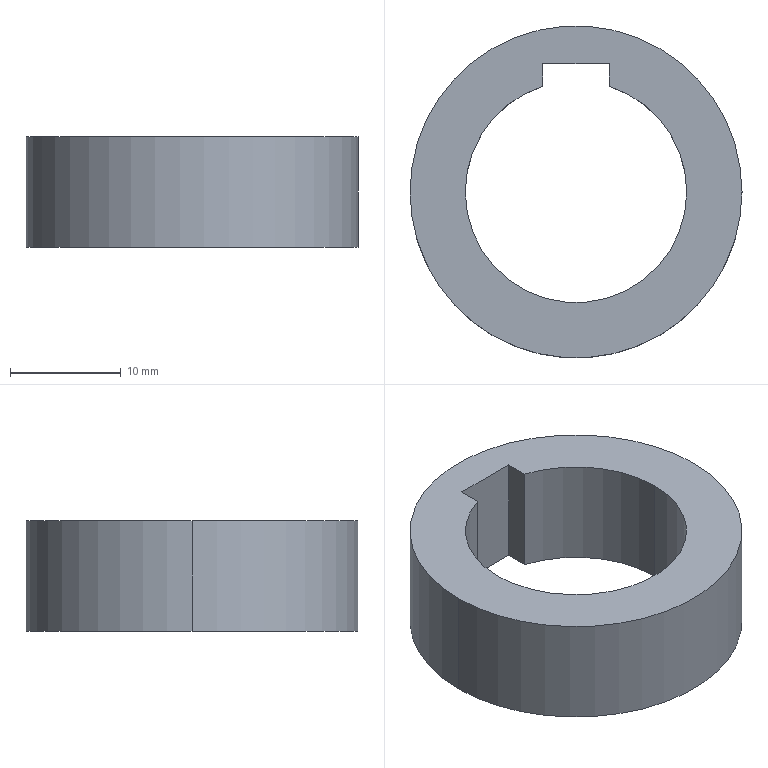Part | SolidWorks | features BaseBody 1 | 1 solid | 10 faces | box 30 x 30 x 10 mm | volume 3822 mm3 | cylinder 5 | plane 5 | commonest cylinder face diameters 20 x3 30 x2
STEP:
#1=CARTESIAN_POINT('',(10.,0.,10.));
#2=VERTEX_POINT('',#1);
#3=CARTESIAN_POINT('',(-10.,0.,10.));
#4=VERTEX_POINT('',#3);
#5=CARTESIAN_POINT('',(0.,0.,10.));
#6=DIRECTION('',(0.,0.,-1.));
#7=DIRECTION('',(-1.,0.,0.));
#8=AXIS2_PLACEMENT_3D('',#5,#6,#7);
#9=CIRCLE('',#8,10.);
#10=EDGE_CURVE('',#2,#4,#9,.T.);
#11=ORIENTED_EDGE('',*,*,#10,.F.);
#12=CARTESIAN_POINT('',(10.,0.,0.));
#13=VERTEX_POINT('',#12);
#14=CARTESIAN_POINT('',(10.,0.,0.));
#15=DIRECTION('',(0.,0.,-1.));
#16=VECTOR('',#15,1000.);
#17=LINE('',#14,#16);
#18=EDGE_CURVE('',#2,#13,#17,.T.);
#19=ORIENTED_EDGE('',*,*,#18,.T.);
#20=CARTESIAN_POINT('',(-10.,0.,0.));
#21=VERTEX_POINT('',#20);
#22=CARTESIAN_POINT('',(0.,0.,0.));
#23=DIRECTION('',(0.,0.,1.));
#24=DIRECTION('',(-1.,0.,0.));
#25=AXIS2_PLACEMENT_3D('',#22,#23,#24);
#26=CIRCLE('',#25,10.);
#27=EDGE_CURVE('',#21,#13,#26,.T.);
#28=ORIENTED_EDGE('',*,*,#27,.F.);
#29=CARTESIAN_POINT('',(-10.,0.,0.));
#30=DIRECTION('',(0.,0.,-1.));
#31=VECTOR('',#30,1000.);
#32=LINE('',#29,#31);
#33=EDGE_CURVE('',#4,#21,#32,.T.);
#34=ORIENTED_EDGE('',*,*,#33,.F.);
#35=EDGE_LOOP('',(#11,#19,#28,#34));
#36=FACE_OUTER_BOUND('',#35,.T.);
#37=CARTESIAN_POINT('',(0.,0.,0.));
#38=DIRECTION('',(0.,0.,-1.));
#39=DIRECTION('',(-1.,0.,0.));
#40=AXIS2_PLACEMENT_3D('',#37,#38,#39);
#41=CYLINDRICAL_SURFACE('',#40,10.);
#42=ADVANCED_FACE('',(#36),#41,.F.);
#43=CARTESIAN_POINT('',(-3.,9.539,10.));
#44=VERTEX_POINT('',#43);
#45=CARTESIAN_POINT('',(0.,0.,10.));
#46=DIRECTION('',(0.,0.,-1.));
#47=DIRECTION('',(-1.,0.,0.));
#48=AXIS2_PLACEMENT_3D('',#45,#46,#47);
#49=CIRCLE('',#48,10.);
#50=EDGE_CURVE('',#4,#44,#49,.T.);
#51=ORIENTED_EDGE('',*,*,#50,.F.);
#52=ORIENTED_EDGE('',*,*,#33,.T.);
#53=CARTESIAN_POINT('',(-3.,9.539,0.));
#54=VERTEX_POINT('',#53);
#55=CARTESIAN_POINT('',(0.,0.,0.));
#56=DIRECTION('',(0.,0.,1.));
#57=DIRECTION('',(-1.,0.,0.));
#58=AXIS2_PLACEMENT_3D('',#55,#56,#57);
#59=CIRCLE('',#58,10.);
#60=EDGE_CURVE('',#54,#21,#59,.T.);
#61=ORIENTED_EDGE('',*,*,#60,.F.);
#62=CARTESIAN_POINT('',(-3.,9.539,0.));
#63=DIRECTION('',(0.,0.,1.));
#64=VECTOR('',#63,1000.);
#65=LINE('',#62,#64);
#66=EDGE_CURVE('',#54,#44,#65,.T.);
#67=ORIENTED_EDGE('',*,*,#66,.T.);
#68=EDGE_LOOP('',(#51,#52,#61,#67));
#69=FACE_OUTER_BOUND('',#68,.T.);
#70=CARTESIAN_POINT('',(0.,0.,0.));
#71=DIRECTION('',(0.,0.,-1.));
#72=DIRECTION('',(-1.,0.,0.));
#73=AXIS2_PLACEMENT_3D('',#70,#71,#72);
#74=CYLINDRICAL_SURFACE('',#73,10.);
#75=ADVANCED_FACE('',(#69),#74,.F.);
#76=CARTESIAN_POINT('',(15.,0.,10.));
#77=VERTEX_POINT('',#76);
#78=CARTESIAN_POINT('',(-15.,0.,10.));
#79=VERTEX_POINT('',#78);
#80=CARTESIAN_POINT('',(0.,0.,10.));
#81=DIRECTION('',(0.,0.,1.));
#82=DIRECTION('',(-1.,0.,0.));
#83=AXIS2_PLACEMENT_3D('',#80,#81,#82);
#84=CIRCLE('',#83,15.);
#85=EDGE_CURVE('',#77,#79,#84,.T.);
#86=ORIENTED_EDGE('',*,*,#85,.F.);
#87=CARTESIAN_POINT('',(15.,0.,0.));
#88=VERTEX_POINT('',#87);
#89=CARTESIAN_POINT('',(15.,0.,0.));
#90=DIRECTION('',(0.,0.,-1.));
#91=VECTOR('',#90,1000.);
#92=LINE('',#89,#91);
#93=EDGE_CURVE('',#77,#88,#92,.T.);
#94=ORIENTED_EDGE('',*,*,#93,.T.);
#95=CARTESIAN_POINT('',(-15.,0.,0.));
#96=VERTEX_POINT('',#95);
#97=CARTESIAN_POINT('',(0.,0.,0.));
#98=DIRECTION('',(0.,0.,-1.));
#99=DIRECTION('',(-1.,0.,0.));
#100=AXIS2_PLACEMENT_3D('',#97,#98,#99);
#101=CIRCLE('',#100,15.);
#102=EDGE_CURVE('',#96,#88,#101,.T.);
#103=ORIENTED_EDGE('',*,*,#102,.F.);
#104=CARTESIAN_POINT('',(-15.,0.,0.));
#105=DIRECTION('',(0.,0.,-1.));
#106=VECTOR('',#105,1000.);
#107=LINE('',#104,#106);
#108=EDGE_CURVE('',#79,#96,#107,.T.);
#109=ORIENTED_EDGE('',*,*,#108,.F.);
#110=EDGE_LOOP('',(#86,#94,#103,#109));
#111=FACE_OUTER_BOUND('',#110,.T.);
#112=CARTESIAN_POINT('',(0.,0.,0.));
#113=DIRECTION('',(0.,0.,-1.));
#114=DIRECTION('',(-1.,0.,0.));
#115=AXIS2_PLACEMENT_3D('',#112,#113,#114);
#116=CYLINDRICAL_SURFACE('',#115,15.);
#117=ADVANCED_FACE('',(#111),#116,.T.);
#118=CARTESIAN_POINT('',(-3.,11.6,10.));
#119=VERTEX_POINT('',#118);
#120=CARTESIAN_POINT('',(3.,11.6,10.));
#121=VERTEX_POINT('',#120);
#122=CARTESIAN_POINT('',(-1.5,11.6,10.));
#123=DIRECTION('',(1.,0.,0.));
#124=VECTOR('',#123,1000.);
#125=LINE('',#122,#124);
#126=EDGE_CURVE('',#119,#121,#125,.T.);
#127=ORIENTED_EDGE('',*,*,#126,.F.);
#128=CARTESIAN_POINT('',(-3.,11.6,0.));
#129=VERTEX_POINT('',#128);
#130=CARTESIAN_POINT('',(-3.,11.6,10.));
#131=DIRECTION('',(0.,0.,-1.));
#132=VECTOR('',#131,1000.);
#133=LINE('',#130,#132);
#134=EDGE_CURVE('',#119,#129,#133,.T.);
#135=ORIENTED_EDGE('',*,*,#134,.T.);
#136=CARTESIAN_POINT('',(3.,11.6,0.));
#137=VERTEX_POINT('',#136);
#138=CARTESIAN_POINT('',(-1.5,11.6,0.));
#139=DIRECTION('',(-1.,0.,0.));
#140=VECTOR('',#139,1000.);
#141=LINE('',#138,#140);
#142=EDGE_CURVE('',#137,#129,#141,.T.);
#143=ORIENTED_EDGE('',*,*,#142,.F.);
#144=CARTESIAN_POINT('',(3.,11.6,10.));
#145=DIRECTION('',(0.,0.,-1.));
#146=VECTOR('',#145,1000.);
#147=LINE('',#144,#146);
#148=EDGE_CURVE('',#121,#137,#147,.T.);
#149=ORIENTED_EDGE('',*,*,#148,.F.);
#150=EDGE_LOOP('',(#127,#135,#143,#149));
#151=FACE_OUTER_BOUND('',#150,.T.);
#152=CARTESIAN_POINT('',(-3.,11.6,10.));
#153=DIRECTION('',(0.,1.,0.));
#154=DIRECTION('',(1.,0.,0.));
#155=AXIS2_PLACEMENT_3D('',#152,#153,#154);
#156=PLANE('',#155);
#157=ADVANCED_FACE('',(#151),#156,.F.);
#158=CARTESIAN_POINT('',(3.,9.539,10.));
#159=VERTEX_POINT('',#158);
#160=CARTESIAN_POINT('',(3.,5.,10.));
#161=DIRECTION('',(0.,-1.,0.));
#162=VECTOR('',#161,1000.);
#163=LINE('',#160,#162);
#164=EDGE_CURVE('',#121,#159,#163,.T.);
#165=ORIENTED_EDGE('',*,*,#164,.F.);
#166=ORIENTED_EDGE('',*,*,#148,.T.);
#167=CARTESIAN_POINT('',(3.,9.539,0.));
#168=VERTEX_POINT('',#167);
#169=CARTESIAN_POINT('',(3.,5.,0.));
#170=DIRECTION('',(0.,1.,0.));
#171=VECTOR('',#170,1000.);
#172=LINE('',#169,#171);
#173=EDGE_CURVE('',#168,#137,#172,.T.);
#174=ORIENTED_EDGE('',*,*,#173,.F.);
#175=CARTESIAN_POINT('',(3.,9.539,0.));
#176=DIRECTION('',(0.,0.,-1.));
#177=VECTOR('',#176,1000.);
#178=LINE('',#175,#177);
#179=EDGE_CURVE('',#159,#168,#178,.T.);
#180=ORIENTED_EDGE('',*,*,#179,.F.);
#181=EDGE_LOOP('',(#165,#166,#174,#180));
#182=FACE_OUTER_BOUND('',#181,.T.);
#183=CARTESIAN_POINT('',(3.,10.,10.));
#184=DIRECTION('',(1.,0.,0.));
#185=DIRECTION('',(0.,1.,0.));
#186=AXIS2_PLACEMENT_3D('',#183,#184,#185);
#187=PLANE('',#186);
#188=ADVANCED_FACE('',(#182),#187,.F.);
#189=CARTESIAN_POINT('',(-3.,4.77,10.));
#190=DIRECTION('',(0.,1.,0.));
#191=VECTOR('',#190,1000.);
#192=LINE('',#189,#191);
#193=EDGE_CURVE('',#44,#119,#192,.T.);
#194=ORIENTED_EDGE('',*,*,#193,.F.);
#195=ORIENTED_EDGE('',*,*,#66,.F.);
#196=CARTESIAN_POINT('',(-3.,4.77,0.));
#197=DIRECTION('',(0.,-1.,0.));
#198=VECTOR('',#197,1000.);
#199=LINE('',#196,#198);
#200=EDGE_CURVE('',#129,#54,#199,.T.);
#201=ORIENTED_EDGE('',*,*,#200,.F.);
#202=ORIENTED_EDGE('',*,*,#134,.F.);
#203=EDGE_LOOP('',(#194,#195,#201,#202));
#204=FACE_OUTER_BOUND('',#203,.T.);
#205=CARTESIAN_POINT('',(-3.,9.539,10.));
#206=DIRECTION('',(-1.,0.,0.));
#207=DIRECTION('',(0.,0.,1.));
#208=AXIS2_PLACEMENT_3D('',#205,#206,#207);
#209=PLANE('',#208);
#210=ADVANCED_FACE('',(#204),#209,.F.);
#211=ORIENTED_EDGE('',*,*,#173,.T.);
#212=ORIENTED_EDGE('',*,*,#142,.T.);
#213=ORIENTED_EDGE('',*,*,#200,.T.);
#214=ORIENTED_EDGE('',*,*,#60,.T.);
#215=ORIENTED_EDGE('',*,*,#27,.T.);
#216=CARTESIAN_POINT('',(0.,0.,0.));
#217=DIRECTION('',(0.,0.,1.));
#218=DIRECTION('',(-1.,0.,0.));
#219=AXIS2_PLACEMENT_3D('',#216,#217,#218);
#220=CIRCLE('',#219,10.);
#221=EDGE_CURVE('',#13,#168,#220,.T.);
#222=ORIENTED_EDGE('',*,*,#221,.T.);
#223=EDGE_LOOP('',(#211,#212,#213,#214,#215,#222));
#224=FACE_BOUND('',#223,.T.);
#225=ORIENTED_EDGE('',*,*,#102,.T.);
#226=CARTESIAN_POINT('',(0.,0.,0.));
#227=DIRECTION('',(0.,0.,-1.));
#228=DIRECTION('',(-1.,0.,0.));
#229=AXIS2_PLACEMENT_3D('',#226,#227,#228);
#230=CIRCLE('',#229,15.);
#231=EDGE_CURVE('',#88,#96,#230,.T.);
#232=ORIENTED_EDGE('',*,*,#231,.T.);
#233=EDGE_LOOP('',(#225,#232));
#234=FACE_OUTER_BOUND('',#233,.T.);
#235=CARTESIAN_POINT('',(0.,0.,0.));
#236=DIRECTION('',(0.,0.,1.));
#237=DIRECTION('',(1.,0.,0.));
#238=AXIS2_PLACEMENT_3D('',#235,#236,#237);
#239=PLANE('',#238);
#240=ADVANCED_FACE('',(#224,#234),#239,.F.);
#241=ORIENTED_EDGE('',*,*,#193,.T.);
#242=ORIENTED_EDGE('',*,*,#126,.T.);
#243=ORIENTED_EDGE('',*,*,#164,.T.);
#244=CARTESIAN_POINT('',(0.,0.,10.));
#245=DIRECTION('',(0.,0.,-1.));
#246=DIRECTION('',(-1.,0.,0.));
#247=AXIS2_PLACEMENT_3D('',#244,#245,#246);
#248=CIRCLE('',#247,10.);
#249=EDGE_CURVE('',#159,#2,#248,.T.);
#250=ORIENTED_EDGE('',*,*,#249,.T.);
#251=ORIENTED_EDGE('',*,*,#10,.T.);
#252=ORIENTED_EDGE('',*,*,#50,.T.);
#253=EDGE_LOOP('',(#241,#242,#243,#250,#251,#252));
#254=FACE_BOUND('',#253,.T.);
#255=CARTESIAN_POINT('',(0.,0.,10.));
#256=DIRECTION('',(0.,0.,1.));
#257=DIRECTION('',(-1.,0.,0.));
#258=AXIS2_PLACEMENT_3D('',#255,#256,#257);
#259=CIRCLE('',#258,15.);
#260=EDGE_CURVE('',#79,#77,#259,.T.);
#261=ORIENTED_EDGE('',*,*,#260,.T.);
#262=ORIENTED_EDGE('',*,*,#85,.T.);
#263=EDGE_LOOP('',(#261,#262));
#264=FACE_OUTER_BOUND('',#263,.T.);
#265=CARTESIAN_POINT('',(0.,0.,10.));
#266=DIRECTION('',(0.,0.,1.));
#267=DIRECTION('',(1.,0.,0.));
#268=AXIS2_PLACEMENT_3D('',#265,#266,#267);
#269=PLANE('',#268);
#270=ADVANCED_FACE('',(#254,#264),#269,.T.);
#271=ORIENTED_EDGE('',*,*,#93,.F.);
#272=ORIENTED_EDGE('',*,*,#260,.F.);
#273=ORIENTED_EDGE('',*,*,#108,.T.);
#274=ORIENTED_EDGE('',*,*,#231,.F.);
#275=EDGE_LOOP('',(#271,#272,#273,#274));
#276=FACE_OUTER_BOUND('',#275,.T.);
#277=CARTESIAN_POINT('',(0.,0.,0.));
#278=DIRECTION('',(0.,0.,-1.));
#279=DIRECTION('',(-1.,0.,0.));
#280=AXIS2_PLACEMENT_3D('',#277,#278,#279);
#281=CYLINDRICAL_SURFACE('',#280,15.);
#282=ADVANCED_FACE('',(#276),#281,.T.);
#283=ORIENTED_EDGE('',*,*,#18,.F.);
#284=ORIENTED_EDGE('',*,*,#249,.F.);
#285=ORIENTED_EDGE('',*,*,#179,.T.);
#286=ORIENTED_EDGE('',*,*,#221,.F.);
#287=EDGE_LOOP('',(#283,#284,#285,#286));
#288=FACE_OUTER_BOUND('',#287,.T.);
#289=CARTESIAN_POINT('',(0.,0.,0.));
#290=DIRECTION('',(0.,0.,-1.));
#291=DIRECTION('',(-1.,0.,0.));
#292=AXIS2_PLACEMENT_3D('',#289,#290,#291);
#293=CYLINDRICAL_SURFACE('',#292,10.);
#294=ADVANCED_FACE('',(#288),#293,.F.);
#295=CLOSED_SHELL('',(#42,#75,#117,#157,#188,#210,#240,#270,#282,#294));
#296=MANIFOLD_SOLID_BREP('',#295);
#297=CARTESIAN_POINT('',(0.,0.,0.));
#298=DIRECTION('',(0.,0.,1.));
#299=DIRECTION('',(1.,0.,0.));
#300=AXIS2_PLACEMENT_3D('',#297,#298,#299);
#301=(LENGTH_UNIT()NAMED_UNIT(*)SI_UNIT(.MILLI.,.METRE.));
#302=UNCERTAINTY_MEASURE_WITH_UNIT(LENGTH_MEASURE(0.00001),#301,'','');
#303=(NAMED_UNIT(*)PLANE_ANGLE_UNIT()SI_UNIT($,.RADIAN.));
#304=(NAMED_UNIT(*)SI_UNIT($,.STERADIAN.)SOLID_ANGLE_UNIT());
#305=(GEOMETRIC_REPRESENTATION_CONTEXT(3)GLOBAL_UNCERTAINTY_ASSIGNED_CONTEXT((#302))GLOBAL_UNIT_ASSIGNED_CONTEXT((#301,#303,#304))REPRESENTATION_CONTEXT('',''));
#306=ADVANCED_BREP_SHAPE_REPRESENTATION('',(#296,#300),#305);